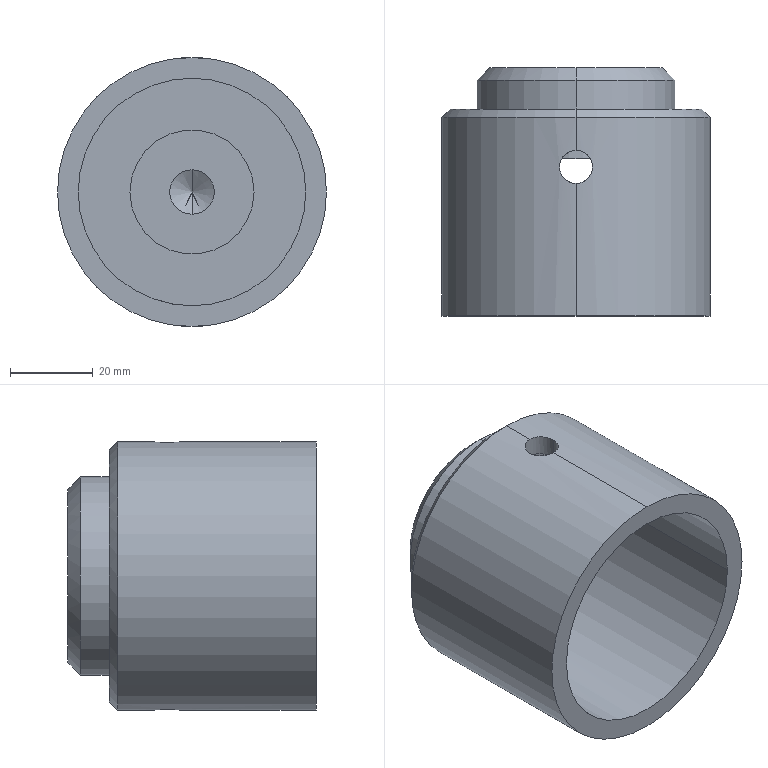Part | SolidWorks | features Chamfer 2, ICE 2, RevCut 2, Revolution 1 | 1 solid | 25 faces | box 65 x 60 x 65 mm | volume 87654 mm3 | cylinder 14 | cone 6 | plane 5 | commonest cylinder face diameters 8 x4 10.75 x2 30 x2 48 x2 55 x2 65 x2
STEP:
#1=CARTESIAN_POINT('',(0.,38.,-5.375));
#2=VERTEX_POINT('',#1);
#3=CARTESIAN_POINT('',(0.,38.,5.375));
#4=VERTEX_POINT('',#3);
#5=CARTESIAN_POINT('',(0.,38.,0.));
#6=DIRECTION('',(0.,1.,0.));
#7=DIRECTION('',(0.,0.,1.));
#8=AXIS2_PLACEMENT_3D('',#5,#6,#7);
#9=CIRCLE('',#8,5.375);
#10=EDGE_CURVE('',#2,#4,#9,.T.);
#11=ORIENTED_EDGE('',*,*,#10,.F.);
#12=CARTESIAN_POINT('',(0.,50.,-5.375));
#13=VERTEX_POINT('',#12);
#14=CARTESIAN_POINT('',(0.,53.103,-5.375));
#15=DIRECTION('',(0.,1.,0.));
#16=VECTOR('',#15,1000.);
#17=LINE('',#14,#16);
#18=EDGE_CURVE('',#2,#13,#17,.T.);
#19=ORIENTED_EDGE('',*,*,#18,.T.);
#20=CARTESIAN_POINT('',(0.,50.,5.375));
#21=VERTEX_POINT('',#20);
#22=CARTESIAN_POINT('',(0.,50.,0.));
#23=DIRECTION('',(0.,1.,0.));
#24=DIRECTION('',(0.,0.,1.));
#25=AXIS2_PLACEMENT_3D('',#22,#23,#24);
#26=CIRCLE('',#25,5.375);
#27=EDGE_CURVE('',#13,#21,#26,.T.);
#28=ORIENTED_EDGE('',*,*,#27,.T.);
#29=CARTESIAN_POINT('',(0.,53.103,5.375));
#30=DIRECTION('',(0.,1.,0.));
#31=VECTOR('',#30,1000.);
#32=LINE('',#29,#31);
#33=EDGE_CURVE('',#4,#21,#32,.T.);
#34=ORIENTED_EDGE('',*,*,#33,.F.);
#35=EDGE_LOOP('',(#11,#19,#28,#34));
#36=FACE_OUTER_BOUND('',#35,.T.);
#37=CARTESIAN_POINT('',(0.,53.103,0.));
#38=DIRECTION('',(0.,1.,0.));
#39=DIRECTION('',(0.,0.,1.));
#40=AXIS2_PLACEMENT_3D('',#37,#38,#39);
#41=CYLINDRICAL_SURFACE('',#40,5.375);
#42=ADVANCED_FACE('',(#36),#41,.F.);
#43=CARTESIAN_POINT('',(0.,53.103,0.));
#44=VERTEX_POINT('',#43);
#45=CARTESIAN_POINT('',(0.,53.103,0.));
#46=DIRECTION('',(0.,-0.5,-0.866));
#47=VECTOR('',#46,1000.);
#48=LINE('',#45,#47);
#49=EDGE_CURVE('',#44,#13,#48,.T.);
#50=ORIENTED_EDGE('',*,*,#49,.F.);
#51=CARTESIAN_POINT('',(0.,53.103,0.));
#52=DIRECTION('',(0.,-0.5,0.866));
#53=VECTOR('',#52,1000.);
#54=LINE('',#51,#53);
#55=EDGE_CURVE('',#44,#21,#54,.T.);
#56=ORIENTED_EDGE('',*,*,#55,.T.);
#57=ORIENTED_EDGE('',*,*,#27,.F.);
#58=EDGE_LOOP('',(#50,#56,#57));
#59=FACE_OUTER_BOUND('',#58,.T.);
#60=CARTESIAN_POINT('',(0.,-946.897,0.));
#61=DIRECTION('',(0.,-1.,0.));
#62=DIRECTION('',(0.,0.,-1.));
#63=AXIS2_PLACEMENT_3D('',#60,#61,#62);
#64=CONICAL_SURFACE('',#63,1732.051,1.047);
#65=ADVANCED_FACE('',(#59),#64,.F.);
#66=CARTESIAN_POINT('',(0.,32.,32.5));
#67=VERTEX_POINT('',#66);
#68=CARTESIAN_POINT('',(4.,36.,32.253));
#69=VERTEX_POINT('',#68);
#70=CARTESIAN_POINT('',(0.,32.,32.5));
#71=CARTESIAN_POINT('',(0.2611,32.,32.5));
#72=CARTESIAN_POINT('',(0.5264,32.026,32.497));
#73=CARTESIAN_POINT('',(1.039,32.129,32.484));
#74=CARTESIAN_POINT('',(1.289,32.204,32.475));
#75=CARTESIAN_POINT('',(1.773,32.405,32.452));
#76=CARTESIAN_POINT('',(2.007,32.53,32.439));
#77=CARTESIAN_POINT('',(2.44,32.82,32.409));
#78=CARTESIAN_POINT('',(2.642,32.985,32.393));
#79=CARTESIAN_POINT('',(3.015,33.358,32.36));
#80=CARTESIAN_POINT('',(3.18,33.56,32.344));
#81=CARTESIAN_POINT('',(3.47,33.993,32.315));
#82=CARTESIAN_POINT('',(3.595,34.227,32.301));
#83=CARTESIAN_POINT('',(3.796,34.711,32.278));
#84=CARTESIAN_POINT('',(3.871,34.961,32.269));
#85=CARTESIAN_POINT('',(3.974,35.474,32.256));
#86=CARTESIAN_POINT('',(4.,35.739,32.253));
#87=CARTESIAN_POINT('',(4.,36.,32.253));
#88=B_SPLINE_CURVE_WITH_KNOTS('',3,(#70,#71,#72,#73,#74,#75,#76,#77,#78,#79,#80,#81,#82,#83,#84,#85,#86,#87),.UNSPECIFIED.,.F.,.F.,(4,2,2,2,2,2,2,2,4),(0.00626,0.007042,0.007825,0.008607,0.009389,0.01017,0.01095,0.01174,0.01252),.UNSPECIFIED.);
#89=EDGE_CURVE('',#67,#69,#88,.T.);
#90=ORIENTED_EDGE('',*,*,#89,.T.);
#91=CARTESIAN_POINT('',(4.,36.,27.208));
#92=VERTEX_POINT('',#91);
#93=CARTESIAN_POINT('',(4.,36.,125.));
#94=DIRECTION('',(0.,0.,-1.));
#95=VECTOR('',#94,1000.);
#96=LINE('',#93,#95);
#97=EDGE_CURVE('',#69,#92,#96,.T.);
#98=ORIENTED_EDGE('',*,*,#97,.T.);
#99=CARTESIAN_POINT('',(-4.,36.,27.208));
#100=VERTEX_POINT('',#99);
#101=CARTESIAN_POINT('',(4.,36.,27.208));
#102=CARTESIAN_POINT('',(4.,35.739,27.208));
#103=CARTESIAN_POINT('',(3.974,35.473,27.211));
#104=CARTESIAN_POINT('',(3.871,34.96,27.226));
#105=CARTESIAN_POINT('',(3.796,34.711,27.237));
#106=CARTESIAN_POINT('',(3.595,34.226,27.264));
#107=CARTESIAN_POINT('',(3.469,33.992,27.281));
#108=CARTESIAN_POINT('',(3.18,33.559,27.316));
#109=CARTESIAN_POINT('',(3.014,33.357,27.335));
#110=CARTESIAN_POINT('',(2.641,32.984,27.374));
#111=CARTESIAN_POINT('',(2.439,32.819,27.392));
#112=CARTESIAN_POINT('',(2.006,32.53,27.428));
#113=CARTESIAN_POINT('',(1.772,32.404,27.444));
#114=CARTESIAN_POINT('',(1.288,32.204,27.471));
#115=CARTESIAN_POINT('',(1.039,32.128,27.482));
#116=CARTESIAN_POINT('',(0.5253,32.026,27.496));
#117=CARTESIAN_POINT('',(0.2599,32.,27.5));
#118=CARTESIAN_POINT('',(-0.2625,32.,27.5));
#119=CARTESIAN_POINT('',(-0.5224,32.026,27.496));
#120=CARTESIAN_POINT('',(-1.039,32.128,27.482));
#121=CARTESIAN_POINT('',(-1.291,32.205,27.471));
#122=CARTESIAN_POINT('',(-1.773,32.405,27.444));
#123=CARTESIAN_POINT('',(-2.006,32.529,27.428));
#124=CARTESIAN_POINT('',(-2.442,32.821,27.392));
#125=CARTESIAN_POINT('',(-2.644,32.987,27.373));
#126=CARTESIAN_POINT('',(-3.012,33.355,27.335));
#127=CARTESIAN_POINT('',(-3.181,33.561,27.316));
#128=CARTESIAN_POINT('',(-3.471,33.995,27.28));
#129=CARTESIAN_POINT('',(-3.594,34.225,27.264));
#130=CARTESIAN_POINT('',(-3.795,34.709,27.237));
#131=CARTESIAN_POINT('',(-3.872,34.963,27.226));
#132=CARTESIAN_POINT('',(-3.974,35.475,27.211));
#133=CARTESIAN_POINT('',(-4.,35.736,27.208));
#134=CARTESIAN_POINT('',(-4.,36.,27.208));
#135=B_SPLINE_CURVE_WITH_KNOTS('',3,(#101,#102,#103,#104,#105,#106,#107,#108,#109,#110,#111,#112,#113,#114,#115,#116,#117,#118,#119,#120,#121,#122,#123,#124,#125,#126,#127,#128,#129,#130,#131,#132,#133,#134),.UNSPECIFIED.,.F.,.F.,(4,2,2,2,2,2,2,2,2,2,2,2,2,2,2,2,4),(0.006263,0.007045,0.007828,0.008611,0.009393,0.01018,0.01096,0.01174,0.01252,0.01331,0.01409,0.01487,0.01565,0.01644,0.01722,0.018,0.01878),.UNSPECIFIED.);
#136=EDGE_CURVE('',#92,#100,#135,.T.);
#137=ORIENTED_EDGE('',*,*,#136,.T.);
#138=CARTESIAN_POINT('',(-4.,36.,32.253));
#139=VERTEX_POINT('',#138);
#140=CARTESIAN_POINT('',(-4.,36.,125.));
#141=DIRECTION('',(0.,0.,-1.));
#142=VECTOR('',#141,1000.);
#143=LINE('',#140,#142);
#144=EDGE_CURVE('',#139,#100,#143,.T.);
#145=ORIENTED_EDGE('',*,*,#144,.F.);
#146=CARTESIAN_POINT('',(-4.,36.,32.253));
#147=CARTESIAN_POINT('',(-4.,35.735,32.253));
#148=CARTESIAN_POINT('',(-3.974,35.475,32.256));
#149=CARTESIAN_POINT('',(-3.872,34.964,32.269));
#150=CARTESIAN_POINT('',(-3.795,34.709,32.278));
#151=CARTESIAN_POINT('',(-3.594,34.225,32.301));
#152=CARTESIAN_POINT('',(-3.471,33.995,32.314));
#153=CARTESIAN_POINT('',(-3.181,33.56,32.344));
#154=CARTESIAN_POINT('',(-3.012,33.355,32.361));
#155=CARTESIAN_POINT('',(-2.643,32.986,32.393));
#156=CARTESIAN_POINT('',(-2.442,32.821,32.409));
#157=CARTESIAN_POINT('',(-2.004,32.528,32.439));
#158=CARTESIAN_POINT('',(-1.772,32.404,32.453));
#159=CARTESIAN_POINT('',(-1.29,32.205,32.475));
#160=CARTESIAN_POINT('',(-1.038,32.128,32.484));
#161=CARTESIAN_POINT('',(-0.521,32.025,32.497));
#162=CARTESIAN_POINT('',(-0.2612,32.,32.5));
#163=CARTESIAN_POINT('',(0.,32.,32.5));
#164=B_SPLINE_CURVE_WITH_KNOTS('',3,(#146,#147,#148,#149,#150,#151,#152,#153,#154,#155,#156,#157,#158,#159,#160,#161,#162,#163),.UNSPECIFIED.,.F.,.F.,(4,2,2,2,2,2,2,2,4),(0.,0.0007825,0.001565,0.002348,0.00313,0.003913,0.004695,0.005478,0.00626),.UNSPECIFIED.);
#165=EDGE_CURVE('',#139,#67,#164,.T.);
#166=ORIENTED_EDGE('',*,*,#165,.T.);
#167=EDGE_LOOP('',(#90,#98,#137,#145,#166));
#168=FACE_OUTER_BOUND('',#167,.T.);
#169=CARTESIAN_POINT('',(0.,36.,125.));
#170=DIRECTION('',(0.,0.,-1.));
#171=DIRECTION('',(-1.,0.,0.));
#172=AXIS2_PLACEMENT_3D('',#169,#170,#171);
#173=CYLINDRICAL_SURFACE('',#172,4.);
#174=ADVANCED_FACE('',(#168),#173,.F.);
#175=CARTESIAN_POINT('',(-4.,36.,-32.253));
#176=VERTEX_POINT('',#175);
#177=CARTESIAN_POINT('',(0.,32.,-32.5));
#178=VERTEX_POINT('',#177);
#179=CARTESIAN_POINT('',(-4.,36.,-32.253));
#180=CARTESIAN_POINT('',(-4.,35.739,-32.253));
#181=CARTESIAN_POINT('',(-3.974,35.474,-32.256));
#182=CARTESIAN_POINT('',(-3.871,34.961,-32.269));
#183=CARTESIAN_POINT('',(-3.796,34.711,-32.278));
#184=CARTESIAN_POINT('',(-3.595,34.227,-32.301));
#185=CARTESIAN_POINT('',(-3.47,33.993,-32.315));
#186=CARTESIAN_POINT('',(-3.18,33.56,-32.344));
#187=CARTESIAN_POINT('',(-3.015,33.358,-32.36));
#188=CARTESIAN_POINT('',(-2.642,32.985,-32.393));
#189=CARTESIAN_POINT('',(-2.44,32.82,-32.409));
#190=CARTESIAN_POINT('',(-2.007,32.53,-32.439));
#191=CARTESIAN_POINT('',(-1.773,32.405,-32.453));
#192=CARTESIAN_POINT('',(-1.289,32.204,-32.475));
#193=CARTESIAN_POINT('',(-1.039,32.129,-32.484));
#194=CARTESIAN_POINT('',(-0.5264,32.026,-32.497));
#195=CARTESIAN_POINT('',(-0.2611,32.,-32.5));
#196=CARTESIAN_POINT('',(0.,32.,-32.5));
#197=B_SPLINE_CURVE_WITH_KNOTS('',3,(#179,#180,#181,#182,#183,#184,#185,#186,#187,#188,#189,#190,#191,#192,#193,#194,#195,#196),.UNSPECIFIED.,.F.,.F.,(4,2,2,2,2,2,2,2,4),(0.00626,0.007042,0.007825,0.008607,0.009389,0.01017,0.01095,0.01174,0.01252),.UNSPECIFIED.);
#198=EDGE_CURVE('',#176,#178,#197,.T.);
#199=ORIENTED_EDGE('',*,*,#198,.F.);
#200=CARTESIAN_POINT('',(-4.,36.,-27.208));
#201=VERTEX_POINT('',#200);
#202=CARTESIAN_POINT('',(-4.,36.,-125.));
#203=DIRECTION('',(0.,0.,1.));
#204=VECTOR('',#203,1000.);
#205=LINE('',#202,#204);
#206=EDGE_CURVE('',#176,#201,#205,.T.);
#207=ORIENTED_EDGE('',*,*,#206,.T.);
#208=CARTESIAN_POINT('',(4.,36.,-27.208));
#209=VERTEX_POINT('',#208);
#210=CARTESIAN_POINT('',(4.,36.,-27.208));
#211=CARTESIAN_POINT('',(4.,35.739,-27.208));
#212=CARTESIAN_POINT('',(3.974,35.473,-27.211));
#213=CARTESIAN_POINT('',(3.871,34.96,-27.226));
#214=CARTESIAN_POINT('',(3.796,34.711,-27.237));
#215=CARTESIAN_POINT('',(3.595,34.226,-27.264));
#216=CARTESIAN_POINT('',(3.469,33.992,-27.281));
#217=CARTESIAN_POINT('',(3.18,33.559,-27.316));
#218=CARTESIAN_POINT('',(3.014,33.357,-27.335));
#219=CARTESIAN_POINT('',(2.641,32.984,-27.374));
#220=CARTESIAN_POINT('',(2.439,32.819,-27.392));
#221=CARTESIAN_POINT('',(2.006,32.53,-27.428));
#222=CARTESIAN_POINT('',(1.772,32.404,-27.444));
#223=CARTESIAN_POINT('',(1.288,32.204,-27.471));
#224=CARTESIAN_POINT('',(1.039,32.128,-27.482));
#225=CARTESIAN_POINT('',(0.5253,32.026,-27.496));
#226=CARTESIAN_POINT('',(0.2599,32.,-27.5));
#227=CARTESIAN_POINT('',(-0.2625,32.,-27.5));
#228=CARTESIAN_POINT('',(-0.5224,32.026,-27.496));
#229=CARTESIAN_POINT('',(-1.039,32.128,-27.482));
#230=CARTESIAN_POINT('',(-1.291,32.205,-27.471));
#231=CARTESIAN_POINT('',(-1.773,32.405,-27.444));
#232=CARTESIAN_POINT('',(-2.006,32.529,-27.428));
#233=CARTESIAN_POINT('',(-2.442,32.821,-27.392));
#234=CARTESIAN_POINT('',(-2.644,32.987,-27.373));
#235=CARTESIAN_POINT('',(-3.012,33.355,-27.335));
#236=CARTESIAN_POINT('',(-3.181,33.561,-27.316));
#237=CARTESIAN_POINT('',(-3.471,33.995,-27.28));
#238=CARTESIAN_POINT('',(-3.594,34.225,-27.264));
#239=CARTESIAN_POINT('',(-3.795,34.709,-27.237));
#240=CARTESIAN_POINT('',(-3.872,34.963,-27.226));
#241=CARTESIAN_POINT('',(-3.974,35.475,-27.211));
#242=CARTESIAN_POINT('',(-4.,35.736,-27.208));
#243=CARTESIAN_POINT('',(-4.,36.,-27.208));
#244=B_SPLINE_CURVE_WITH_KNOTS('',3,(#210,#211,#212,#213,#214,#215,#216,#217,#218,#219,#220,#221,#222,#223,#224,#225,#226,#227,#228,#229,#230,#231,#232,#233,#234,#235,#236,#237,#238,#239,#240,#241,#242,#243),.UNSPECIFIED.,.F.,.F.,(4,2,2,2,2,2,2,2,2,2,2,2,2,2,2,2,4),(0.006263,0.007045,0.007828,0.008611,0.009393,0.01018,0.01096,0.01174,0.01252,0.01331,0.01409,0.01487,0.01565,0.01644,0.01722,0.018,0.01878),.UNSPECIFIED.);
#245=EDGE_CURVE('',#209,#201,#244,.T.);
#246=ORIENTED_EDGE('',*,*,#245,.F.);
#247=CARTESIAN_POINT('',(4.,36.,-32.253));
#248=VERTEX_POINT('',#247);
#249=CARTESIAN_POINT('',(4.,36.,-125.));
#250=DIRECTION('',(0.,0.,1.));
#251=VECTOR('',#250,1000.);
#252=LINE('',#249,#251);
#253=EDGE_CURVE('',#248,#209,#252,.T.);
#254=ORIENTED_EDGE('',*,*,#253,.F.);
#255=CARTESIAN_POINT('',(0.,32.,-32.5));
#256=CARTESIAN_POINT('',(0.2612,32.,-32.5));
#257=CARTESIAN_POINT('',(0.5211,32.025,-32.497));
#258=CARTESIAN_POINT('',(1.038,32.128,-32.484));
#259=CARTESIAN_POINT('',(1.29,32.205,-32.475));
#260=CARTESIAN_POINT('',(1.772,32.404,-32.453));
#261=CARTESIAN_POINT('',(2.005,32.529,-32.439));
#262=CARTESIAN_POINT('',(2.442,32.821,-32.409));
#263=CARTESIAN_POINT('',(2.643,32.986,-32.393));
#264=CARTESIAN_POINT('',(3.012,33.355,-32.361));
#265=CARTESIAN_POINT('',(3.181,33.561,-32.344));
#266=CARTESIAN_POINT('',(3.471,33.995,-32.314));
#267=CARTESIAN_POINT('',(3.594,34.225,-32.301));
#268=CARTESIAN_POINT('',(3.795,34.709,-32.278));
#269=CARTESIAN_POINT('',(3.872,34.964,-32.269));
#270=CARTESIAN_POINT('',(3.974,35.475,-32.256));
#271=CARTESIAN_POINT('',(4.,35.735,-32.253));
#272=CARTESIAN_POINT('',(4.,36.,-32.253));
#273=B_SPLINE_CURVE_WITH_KNOTS('',3,(#255,#256,#257,#258,#259,#260,#261,#262,#263,#264,#265,#266,#267,#268,#269,#270,#271,#272),.UNSPECIFIED.,.F.,.F.,(4,2,2,2,2,2,2,2,4),(0.01252,0.0133,0.01408,0.01487,0.01565,0.01643,0.01721,0.018,0.01878),.UNSPECIFIED.);
#274=EDGE_CURVE('',#178,#248,#273,.T.);
#275=ORIENTED_EDGE('',*,*,#274,.F.);
#276=EDGE_LOOP('',(#199,#207,#246,#254,#275));
#277=FACE_OUTER_BOUND('',#276,.T.);
#278=CARTESIAN_POINT('',(0.,36.,-125.));
#279=DIRECTION('',(0.,0.,1.));
#280=DIRECTION('',(1.,0.,0.));
#281=AXIS2_PLACEMENT_3D('',#278,#279,#280);
#282=CYLINDRICAL_SURFACE('',#281,4.);
#283=ADVANCED_FACE('',(#277),#282,.F.);
#284=CARTESIAN_POINT('',(-15.,38.,0.));
#285=VERTEX_POINT('',#284);
#286=CARTESIAN_POINT('',(15.,38.,0.));
#287=VERTEX_POINT('',#286);
#288=CARTESIAN_POINT('',(0.,38.,0.));
#289=DIRECTION('',(0.,1.,0.));
#290=DIRECTION('',(-1.,0.,0.));
#291=AXIS2_PLACEMENT_3D('',#288,#289,#290);
#292=CIRCLE('',#291,15.);
#293=EDGE_CURVE('',#285,#287,#292,.T.);
#294=ORIENTED_EDGE('',*,*,#293,.T.);
#295=CARTESIAN_POINT('',(15.,40.,0.));
#296=VERTEX_POINT('',#295);
#297=CARTESIAN_POINT('',(15.,38.,0.));
#298=DIRECTION('',(0.,1.,0.));
#299=VECTOR('',#298,1000.);
#300=LINE('',#297,#299);
#301=EDGE_CURVE('',#287,#296,#300,.T.);
#302=ORIENTED_EDGE('',*,*,#301,.T.);
#303=CARTESIAN_POINT('',(-15.,40.,0.));
#304=VERTEX_POINT('',#303);
#305=CARTESIAN_POINT('',(0.,40.,0.));
#306=DIRECTION('',(0.,1.,0.));
#307=DIRECTION('',(-1.,0.,0.));
#308=AXIS2_PLACEMENT_3D('',#305,#306,#307);
#309=CIRCLE('',#308,15.);
#310=EDGE_CURVE('',#304,#296,#309,.T.);
#311=ORIENTED_EDGE('',*,*,#310,.F.);
#312=CARTESIAN_POINT('',(-15.,38.,0.));
#313=DIRECTION('',(0.,1.,0.));
#314=VECTOR('',#313,1000.);
#315=LINE('',#312,#314);
#316=EDGE_CURVE('',#285,#304,#315,.T.);
#317=ORIENTED_EDGE('',*,*,#316,.F.);
#318=EDGE_LOOP('',(#294,#302,#311,#317));
#319=FACE_OUTER_BOUND('',#318,.T.);
#320=CARTESIAN_POINT('',(0.,38.,0.));
#321=DIRECTION('',(0.,1.,0.));
#322=DIRECTION('',(-1.,0.,0.));
#323=AXIS2_PLACEMENT_3D('',#320,#321,#322);
#324=CYLINDRICAL_SURFACE('',#323,15.);
#325=ADVANCED_FACE('',(#319),#324,.T.);
#326=CARTESIAN_POINT('',(0.,50.,30.5));
#327=VERTEX_POINT('',#326);
#328=CARTESIAN_POINT('',(0.,50.,-30.5));
#329=VERTEX_POINT('',#328);
#330=CARTESIAN_POINT('',(0.,50.,0.));
#331=DIRECTION('',(0.,1.,0.));
#332=DIRECTION('',(0.,0.,-1.));
#333=AXIS2_PLACEMENT_3D('',#330,#331,#332);
#334=CIRCLE('',#333,30.5);
#335=EDGE_CURVE('',#327,#329,#334,.T.);
#336=ORIENTED_EDGE('',*,*,#335,.F.);
#337=CARTESIAN_POINT('',(0.,48.,32.5));
#338=VERTEX_POINT('',#337);
#339=CARTESIAN_POINT('',(0.,48.,32.5));
#340=DIRECTION('',(0.,-0.7071,0.7071));
#341=VECTOR('',#340,1000.);
#342=LINE('',#339,#341);
#343=EDGE_CURVE('',#327,#338,#342,.T.);
#344=ORIENTED_EDGE('',*,*,#343,.T.);
#345=CARTESIAN_POINT('',(0.,48.,-32.5));
#346=VERTEX_POINT('',#345);
#347=CARTESIAN_POINT('',(0.,48.,0.));
#348=DIRECTION('',(0.,-1.,0.));
#349=DIRECTION('',(0.,0.,-1.));
#350=AXIS2_PLACEMENT_3D('',#347,#348,#349);
#351=CIRCLE('',#350,32.5);
#352=EDGE_CURVE('',#346,#338,#351,.T.);
#353=ORIENTED_EDGE('',*,*,#352,.F.);
#354=CARTESIAN_POINT('',(0.,48.,-32.5));
#355=DIRECTION('',(0.,-0.7071,-0.7071));
#356=VECTOR('',#355,1000.);
#357=LINE('',#354,#356);
#358=EDGE_CURVE('',#329,#346,#357,.T.);
#359=ORIENTED_EDGE('',*,*,#358,.F.);
#360=EDGE_LOOP('',(#336,#344,#353,#359));
#361=FACE_OUTER_BOUND('',#360,.T.);
#362=CARTESIAN_POINT('',(0.,48.,0.));
#363=DIRECTION('',(0.,-1.,0.));
#364=DIRECTION('',(0.,0.,-1.));
#365=AXIS2_PLACEMENT_3D('',#362,#363,#364);
#366=CONICAL_SURFACE('',#365,32.5,0.7854);
#367=ADVANCED_FACE('',(#361),#366,.T.);
#368=CARTESIAN_POINT('',(0.,60.,21.));
#369=VERTEX_POINT('',#368);
#370=CARTESIAN_POINT('',(0.,60.,-21.));
#371=VERTEX_POINT('',#370);
#372=CARTESIAN_POINT('',(0.,60.,0.));
#373=DIRECTION('',(0.,1.,0.));
#374=DIRECTION('',(0.,0.,-1.));
#375=AXIS2_PLACEMENT_3D('',#372,#373,#374);
#376=CIRCLE('',#375,21.);
#377=EDGE_CURVE('',#369,#371,#376,.T.);
#378=ORIENTED_EDGE('',*,*,#377,.F.);
#379=CARTESIAN_POINT('',(0.,57.,24.));
#380=VERTEX_POINT('',#379);
#381=CARTESIAN_POINT('',(0.,57.,24.));
#382=DIRECTION('',(0.,-0.7071,0.7071));
#383=VECTOR('',#382,1000.);
#384=LINE('',#381,#383);
#385=EDGE_CURVE('',#369,#380,#384,.T.);
#386=ORIENTED_EDGE('',*,*,#385,.T.);
#387=CARTESIAN_POINT('',(0.,57.,-24.));
#388=VERTEX_POINT('',#387);
#389=CARTESIAN_POINT('',(0.,57.,0.));
#390=DIRECTION('',(0.,-1.,0.));
#391=DIRECTION('',(0.,0.,-1.));
#392=AXIS2_PLACEMENT_3D('',#389,#390,#391);
#393=CIRCLE('',#392,24.);
#394=EDGE_CURVE('',#388,#380,#393,.T.);
#395=ORIENTED_EDGE('',*,*,#394,.F.);
#396=CARTESIAN_POINT('',(0.,57.,-24.));
#397=DIRECTION('',(0.,-0.7071,-0.7071));
#398=VECTOR('',#397,1000.);
#399=LINE('',#396,#398);
#400=EDGE_CURVE('',#371,#388,#399,.T.);
#401=ORIENTED_EDGE('',*,*,#400,.F.);
#402=EDGE_LOOP('',(#378,#386,#395,#401));
#403=FACE_OUTER_BOUND('',#402,.T.);
#404=CARTESIAN_POINT('',(0.,57.,0.));
#405=DIRECTION('',(0.,-1.,0.));
#406=DIRECTION('',(0.,0.,-1.));
#407=AXIS2_PLACEMENT_3D('',#404,#405,#406);
#408=CONICAL_SURFACE('',#407,24.,0.7854);
#409=ADVANCED_FACE('',(#403),#408,.T.);
#410=ORIENTED_EDGE('',*,*,#394,.T.);
#411=CARTESIAN_POINT('',(0.,50.,24.));
#412=VERTEX_POINT('',#411);
#413=CARTESIAN_POINT('',(0.,0.,24.));
#414=DIRECTION('',(0.,-1.,0.));
#415=VECTOR('',#414,1000.);
#416=LINE('',#413,#415);
#417=EDGE_CURVE('',#380,#412,#416,.T.);
#418=ORIENTED_EDGE('',*,*,#417,.T.);
#419=CARTESIAN_POINT('',(0.,50.,-24.));
#420=VERTEX_POINT('',#419);
#421=CARTESIAN_POINT('',(0.,50.,0.));
#422=DIRECTION('',(0.,-1.,0.));
#423=DIRECTION('',(0.,0.,-1.));
#424=AXIS2_PLACEMENT_3D('',#421,#422,#423);
#425=CIRCLE('',#424,24.);
#426=EDGE_CURVE('',#420,#412,#425,.T.);
#427=ORIENTED_EDGE('',*,*,#426,.F.);
#428=CARTESIAN_POINT('',(0.,0.,-24.));
#429=DIRECTION('',(0.,-1.,0.));
#430=VECTOR('',#429,1000.);
#431=LINE('',#428,#430);
#432=EDGE_CURVE('',#388,#420,#431,.T.);
#433=ORIENTED_EDGE('',*,*,#432,.F.);
#434=EDGE_LOOP('',(#410,#418,#427,#433));
#435=FACE_OUTER_BOUND('',#434,.T.);
#436=CARTESIAN_POINT('',(0.,0.,0.));
#437=DIRECTION('',(0.,-1.,0.));
#438=DIRECTION('',(0.,0.,-1.));
#439=AXIS2_PLACEMENT_3D('',#436,#437,#438);
#440=CYLINDRICAL_SURFACE('',#439,24.);
#441=ADVANCED_FACE('',(#435),#440,.T.);
#442=CARTESIAN_POINT('',(27.5,0.,0.));
#443=VERTEX_POINT('',#442);
#444=CARTESIAN_POINT('',(-27.5,0.,0.));
#445=VERTEX_POINT('',#444);
#446=CARTESIAN_POINT('',(0.,0.,0.));
#447=DIRECTION('',(0.,1.,0.));
#448=DIRECTION('',(-1.,0.,0.));
#449=AXIS2_PLACEMENT_3D('',#446,#447,#448);
#450=CIRCLE('',#449,27.5);
#451=EDGE_CURVE('',#443,#445,#450,.T.);
#452=ORIENTED_EDGE('',*,*,#451,.F.);
#453=CARTESIAN_POINT('',(27.5,40.,0.));
#454=VERTEX_POINT('',#453);
#455=CARTESIAN_POINT('',(27.5,38.,0.));
#456=DIRECTION('',(0.,1.,0.));
#457=VECTOR('',#456,1000.);
#458=LINE('',#455,#457);
#459=EDGE_CURVE('',#443,#454,#458,.T.);
#460=ORIENTED_EDGE('',*,*,#459,.T.);
#461=CARTESIAN_POINT('',(0.,40.,-27.5));
#462=VERTEX_POINT('',#461);
#463=CARTESIAN_POINT('',(0.,40.,0.));
#464=DIRECTION('',(0.,1.,0.));
#465=DIRECTION('',(-1.,0.,0.));
#466=AXIS2_PLACEMENT_3D('',#463,#464,#465);
#467=CIRCLE('',#466,27.5);
#468=EDGE_CURVE('',#454,#462,#467,.T.);
#469=ORIENTED_EDGE('',*,*,#468,.T.);
#470=CARTESIAN_POINT('',(0.,40.,-27.5));
#471=CARTESIAN_POINT('',(0.2647,40.,-27.5));
#472=CARTESIAN_POINT('',(0.525,39.974,-27.496));
#473=CARTESIAN_POINT('',(1.037,39.872,-27.482));
#474=CARTESIAN_POINT('',(1.291,39.795,-27.471));
#475=CARTESIAN_POINT('',(1.776,39.594,-27.444));
#476=CARTESIAN_POINT('',(2.005,39.471,-27.428));
#477=CARTESIAN_POINT('',(2.44,39.18,-27.392));
#478=CARTESIAN_POINT('',(2.645,39.012,-27.373));
#479=CARTESIAN_POINT('',(3.014,38.643,-27.335));
#480=CARTESIAN_POINT('',(3.179,38.442,-27.316));
#481=CARTESIAN_POINT('',(3.472,38.004,-27.28));
#482=CARTESIAN_POINT('',(3.596,37.772,-27.264));
#483=CARTESIAN_POINT('',(3.795,37.29,-27.237));
#484=CARTESIAN_POINT('',(3.872,37.038,-27.226));
#485=CARTESIAN_POINT('',(3.975,36.521,-27.211));
#486=CARTESIAN_POINT('',(4.,36.261,-27.208));
#487=CARTESIAN_POINT('',(4.,36.,-27.208));
#488=B_SPLINE_CURVE_WITH_KNOTS('',3,(#470,#471,#472,#473,#474,#475,#476,#477,#478,#479,#480,#481,#482,#483,#484,#485,#486,#487),.UNSPECIFIED.,.F.,.F.,(4,2,2,2,2,2,2,2,4),(0.,0.0007828,0.001566,0.002349,0.003131,0.003914,0.004697,0.00548,0.006263),.UNSPECIFIED.);
#489=EDGE_CURVE('',#462,#209,#488,.T.);
#490=ORIENTED_EDGE('',*,*,#489,.T.);
#491=ORIENTED_EDGE('',*,*,#245,.T.);
#492=CARTESIAN_POINT('',(-4.,36.,-27.208));
#493=CARTESIAN_POINT('',(-4.,36.264,-27.208));
#494=CARTESIAN_POINT('',(-3.974,36.524,-27.211));
#495=CARTESIAN_POINT('',(-3.872,37.036,-27.226));
#496=CARTESIAN_POINT('',(-3.795,37.29,-27.237));
#497=CARTESIAN_POINT('',(-3.595,37.774,-27.264));
#498=CARTESIAN_POINT('',(-3.472,38.003,-27.28));
#499=CARTESIAN_POINT('',(-3.182,38.438,-27.316));
#500=CARTESIAN_POINT('',(-3.013,38.643,-27.335));
#501=CARTESIAN_POINT('',(-2.645,39.012,-27.373));
#502=CARTESIAN_POINT('',(-2.444,39.177,-27.392));
#503=CARTESIAN_POINT('',(-2.007,39.47,-27.428));
#504=CARTESIAN_POINT('',(-1.776,39.594,-27.444));
#505=CARTESIAN_POINT('',(-1.295,39.794,-27.471));
#506=CARTESIAN_POINT('',(-1.043,39.871,-27.481));
#507=CARTESIAN_POINT('',(-0.5259,39.974,-27.496));
#508=CARTESIAN_POINT('',(-0.2645,40.,-27.5));
#509=CARTESIAN_POINT('',(0.,40.,-27.5));
#510=B_SPLINE_CURVE_WITH_KNOTS('',3,(#492,#493,#494,#495,#496,#497,#498,#499,#500,#501,#502,#503,#504,#505,#506,#507,#508,#509),.UNSPECIFIED.,.F.,.F.,(4,2,2,2,2,2,2,2,4),(0.01878,0.01957,0.02035,0.02113,0.02191,0.0227,0.02348,0.02426,0.02504),.UNSPECIFIED.);
#511=EDGE_CURVE('',#201,#462,#510,.T.);
#512=ORIENTED_EDGE('',*,*,#511,.T.);
#513=CARTESIAN_POINT('',(-27.5,40.,0.));
#514=VERTEX_POINT('',#513);
#515=CARTESIAN_POINT('',(0.,40.,0.));
#516=DIRECTION('',(0.,1.,0.));
#517=DIRECTION('',(-1.,0.,0.));
#518=AXIS2_PLACEMENT_3D('',#515,#516,#517);
#519=CIRCLE('',#518,27.5);
#520=EDGE_CURVE('',#462,#514,#519,.T.);
#521=ORIENTED_EDGE('',*,*,#520,.T.);
#522=CARTESIAN_POINT('',(-27.5,38.,0.));
#523=DIRECTION('',(0.,1.,0.));
#524=VECTOR('',#523,1000.);
#525=LINE('',#522,#524);
#526=EDGE_CURVE('',#445,#514,#525,.T.);
#527=ORIENTED_EDGE('',*,*,#526,.F.);
#528=EDGE_LOOP('',(#452,#460,#469,#490,#491,#512,#521,#527));
#529=FACE_OUTER_BOUND('',#528,.T.);
#530=CARTESIAN_POINT('',(0.,38.,0.));
#531=DIRECTION('',(0.,1.,0.));
#532=DIRECTION('',(-1.,0.,0.));
#533=AXIS2_PLACEMENT_3D('',#530,#531,#532);
#534=CYLINDRICAL_SURFACE('',#533,27.5);
#535=ADVANCED_FACE('',(#529),#534,.F.);
#536=ORIENTED_EDGE('',*,*,#352,.T.);
#537=CARTESIAN_POINT('',(0.,40.,32.5));
#538=VERTEX_POINT('',#537);
#539=CARTESIAN_POINT('',(0.,0.,32.5));
#540=DIRECTION('',(0.,-1.,0.));
#541=VECTOR('',#540,1000.);
#542=LINE('',#539,#541);
#543=EDGE_CURVE('',#338,#538,#542,.T.);
#544=ORIENTED_EDGE('',*,*,#543,.T.);
#545=CARTESIAN_POINT('',(4.,36.,32.253));
#546=CARTESIAN_POINT('',(4.,36.261,32.253));
#547=CARTESIAN_POINT('',(3.975,36.521,32.256));
#548=CARTESIAN_POINT('',(3.872,37.038,32.269));
#549=CARTESIAN_POINT('',(3.795,37.29,32.278));
#550=CARTESIAN_POINT('',(3.596,37.772,32.301));
#551=CARTESIAN_POINT('',(3.471,38.005,32.314));
#552=CARTESIAN_POINT('',(3.179,38.442,32.344));
#553=CARTESIAN_POINT('',(3.014,38.643,32.36));
#554=CARTESIAN_POINT('',(2.645,39.012,32.393));
#555=CARTESIAN_POINT('',(2.439,39.181,32.409));
#556=CARTESIAN_POINT('',(2.005,39.471,32.439));
#557=CARTESIAN_POINT('',(1.775,39.594,32.452));
#558=CARTESIAN_POINT('',(1.291,39.795,32.475));
#559=CARTESIAN_POINT('',(1.036,39.872,32.484));
#560=CARTESIAN_POINT('',(0.5248,39.974,32.497));
#561=CARTESIAN_POINT('',(0.2646,40.,32.5));
#562=CARTESIAN_POINT('',(0.,40.,32.5));
#563=B_SPLINE_CURVE_WITH_KNOTS('',3,(#545,#546,#547,#548,#549,#550,#551,#552,#553,#554,#555,#556,#557,#558,#559,#560,#561,#562),.UNSPECIFIED.,.F.,.F.,(4,2,2,2,2,2,2,2,4),(0.01252,0.0133,0.01408,0.01487,0.01565,0.01643,0.01721,0.018,0.01878),.UNSPECIFIED.);
#564=EDGE_CURVE('',#69,#538,#563,.T.);
#565=ORIENTED_EDGE('',*,*,#564,.F.);
#566=ORIENTED_EDGE('',*,*,#89,.F.);
#567=CARTESIAN_POINT('',(0.,0.,32.5));
#568=VERTEX_POINT('',#567);
#569=CARTESIAN_POINT('',(0.,0.,32.5));
#570=DIRECTION('',(0.,-1.,0.));
#571=VECTOR('',#570,1000.);
#572=LINE('',#569,#571);
#573=EDGE_CURVE('',#67,#568,#572,.T.);
#574=ORIENTED_EDGE('',*,*,#573,.T.);
#575=CARTESIAN_POINT('',(0.,0.,-32.5));
#576=VERTEX_POINT('',#575);
#577=CARTESIAN_POINT('',(0.,0.,0.));
#578=DIRECTION('',(0.,-1.,0.));
#579=DIRECTION('',(0.,0.,-1.));
#580=AXIS2_PLACEMENT_3D('',#577,#578,#579);
#581=CIRCLE('',#580,32.5);
#582=EDGE_CURVE('',#576,#568,#581,.T.);
#583=ORIENTED_EDGE('',*,*,#582,.F.);
#584=CARTESIAN_POINT('',(0.,0.,-32.5));
#585=DIRECTION('',(0.,-1.,0.));
#586=VECTOR('',#585,1000.);
#587=LINE('',#584,#586);
#588=EDGE_CURVE('',#178,#576,#587,.T.);
#589=ORIENTED_EDGE('',*,*,#588,.F.);
#590=ORIENTED_EDGE('',*,*,#274,.T.);
#591=CARTESIAN_POINT('',(0.,40.,-32.5));
#592=VERTEX_POINT('',#591);
#593=CARTESIAN_POINT('',(4.,36.,-32.253));
#594=CARTESIAN_POINT('',(4.,36.264,-32.253));
#595=CARTESIAN_POINT('',(3.974,36.524,-32.256));
#596=CARTESIAN_POINT('',(3.872,37.036,-32.269));
#597=CARTESIAN_POINT('',(3.795,37.29,-32.278));
#598=CARTESIAN_POINT('',(3.595,37.774,-32.301));
#599=CARTESIAN_POINT('',(3.472,38.003,-32.314));
#600=CARTESIAN_POINT('',(3.182,38.438,-32.344));
#601=CARTESIAN_POINT('',(3.013,38.643,-32.361));
#602=CARTESIAN_POINT('',(2.645,39.012,-32.393));
#603=CARTESIAN_POINT('',(2.444,39.177,-32.409));
#604=CARTESIAN_POINT('',(2.007,39.47,-32.439));
#605=CARTESIAN_POINT('',(1.775,39.594,-32.452));
#606=CARTESIAN_POINT('',(1.294,39.794,-32.475));
#607=CARTESIAN_POINT('',(1.043,39.871,-32.484));
#608=CARTESIAN_POINT('',(0.5257,39.974,-32.497));
#609=CARTESIAN_POINT('',(0.2644,40.,-32.5));
#610=CARTESIAN_POINT('',(0.,40.,-32.5));
#611=B_SPLINE_CURVE_WITH_KNOTS('',3,(#593,#594,#595,#596,#597,#598,#599,#600,#601,#602,#603,#604,#605,#606,#607,#608,#609,#610),.UNSPECIFIED.,.F.,.F.,(4,2,2,2,2,2,2,2,4),(0.01878,0.01956,0.02034,0.02112,0.02191,0.02269,0.02347,0.02425,0.02503),.UNSPECIFIED.);
#612=EDGE_CURVE('',#248,#592,#611,.T.);
#613=ORIENTED_EDGE('',*,*,#612,.T.);
#614=CARTESIAN_POINT('',(0.,0.,-32.5));
#615=DIRECTION('',(0.,-1.,0.));
#616=VECTOR('',#615,1000.);
#617=LINE('',#614,#616);
#618=EDGE_CURVE('',#346,#592,#617,.T.);
#619=ORIENTED_EDGE('',*,*,#618,.F.);
#620=EDGE_LOOP('',(#536,#544,#565,#566,#574,#583,#589,#590,#613,#619));
#621=FACE_OUTER_BOUND('',#620,.T.);
#622=CARTESIAN_POINT('',(0.,0.,0.));
#623=DIRECTION('',(0.,-1.,0.));
#624=DIRECTION('',(0.,0.,-1.));
#625=AXIS2_PLACEMENT_3D('',#622,#623,#624);
#626=CYLINDRICAL_SURFACE('',#625,32.5);
#627=ADVANCED_FACE('',(#621),#626,.T.);
#628=ORIENTED_EDGE('',*,*,#543,.F.);
#629=CARTESIAN_POINT('',(0.,48.,0.));
#630=DIRECTION('',(0.,-1.,0.));
#631=DIRECTION('',(0.,0.,-1.));
#632=AXIS2_PLACEMENT_3D('',#629,#630,#631);
#633=CIRCLE('',#632,32.5);
#634=EDGE_CURVE('',#338,#346,#633,.T.);
#635=ORIENTED_EDGE('',*,*,#634,.T.);
#636=ORIENTED_EDGE('',*,*,#618,.T.);
#637=CARTESIAN_POINT('',(0.,40.,-32.5));
#638=CARTESIAN_POINT('',(-0.2646,40.,-32.5));
#639=CARTESIAN_POINT('',(-0.5248,39.974,-32.497));
#640=CARTESIAN_POINT('',(-1.036,39.872,-32.484));
#641=CARTESIAN_POINT('',(-1.291,39.795,-32.475));
#642=CARTESIAN_POINT('',(-1.775,39.594,-32.452));
#643=CARTESIAN_POINT('',(-2.005,39.471,-32.439));
#644=CARTESIAN_POINT('',(-2.44,39.181,-32.409));
#645=CARTESIAN_POINT('',(-2.645,39.012,-32.393));
#646=CARTESIAN_POINT('',(-3.014,38.643,-32.36));
#647=CARTESIAN_POINT('',(-3.179,38.442,-32.344));
#648=CARTESIAN_POINT('',(-3.472,38.004,-32.314));
#649=CARTESIAN_POINT('',(-3.596,37.772,-32.301));
#650=CARTESIAN_POINT('',(-3.795,37.29,-32.278));
#651=CARTESIAN_POINT('',(-3.872,37.038,-32.269));
#652=CARTESIAN_POINT('',(-3.975,36.521,-32.256));
#653=CARTESIAN_POINT('',(-4.,36.261,-32.253));
#654=CARTESIAN_POINT('',(-4.,36.,-32.253));
#655=B_SPLINE_CURVE_WITH_KNOTS('',3,(#637,#638,#639,#640,#641,#642,#643,#644,#645,#646,#647,#648,#649,#650,#651,#652,#653,#654),.UNSPECIFIED.,.F.,.F.,(4,2,2,2,2,2,2,2,4),(0.,0.0007825,0.001565,0.002348,0.00313,0.003913,0.004695,0.005478,0.00626),.UNSPECIFIED.);
#656=EDGE_CURVE('',#592,#176,#655,.T.);
#657=ORIENTED_EDGE('',*,*,#656,.T.);
#658=ORIENTED_EDGE('',*,*,#198,.T.);
#659=ORIENTED_EDGE('',*,*,#588,.T.);
#660=CARTESIAN_POINT('',(0.,0.,0.));
#661=DIRECTION('',(0.,-1.,0.));
#662=DIRECTION('',(0.,0.,-1.));
#663=AXIS2_PLACEMENT_3D('',#660,#661,#662);
#664=CIRCLE('',#663,32.5);
#665=EDGE_CURVE('',#568,#576,#664,.T.);
#666=ORIENTED_EDGE('',*,*,#665,.F.);
#667=ORIENTED_EDGE('',*,*,#573,.F.);
#668=ORIENTED_EDGE('',*,*,#165,.F.);
#669=CARTESIAN_POINT('',(0.,40.,32.5));
#670=CARTESIAN_POINT('',(-0.2643,40.,32.5));
#671=CARTESIAN_POINT('',(-0.5242,39.974,32.497));
#672=CARTESIAN_POINT('',(-1.036,39.872,32.485));
#673=CARTESIAN_POINT('',(-1.29,39.795,32.475));
#674=CARTESIAN_POINT('',(-1.774,39.595,32.452));
#675=CARTESIAN_POINT('',(-2.003,39.472,32.439));
#676=CARTESIAN_POINT('',(-2.438,39.182,32.409));
#677=CARTESIAN_POINT('',(-2.643,39.013,32.393));
#678=CARTESIAN_POINT('',(-3.012,38.645,32.361));
#679=CARTESIAN_POINT('',(-3.177,38.444,32.345));
#680=CARTESIAN_POINT('',(-3.47,38.007,32.315));
#681=CARTESIAN_POINT('',(-3.594,37.775,32.301));
#682=CARTESIAN_POINT('',(-3.794,37.294,32.278));
#683=CARTESIAN_POINT('',(-3.871,37.043,32.269));
#684=CARTESIAN_POINT('',(-3.974,36.526,32.256));
#685=CARTESIAN_POINT('',(-4.,36.264,32.253));
#686=CARTESIAN_POINT('',(-4.,36.,32.253));
#687=B_SPLINE_CURVE_WITH_KNOTS('',3,(#669,#670,#671,#672,#673,#674,#675,#676,#677,#678,#679,#680,#681,#682,#683,#684,#685,#686),.UNSPECIFIED.,.F.,.F.,(4,2,2,2,2,2,2,2,4),(0.01878,0.01956,0.02034,0.02112,0.02191,0.02269,0.02347,0.02425,0.02503),.UNSPECIFIED.);
#688=EDGE_CURVE('',#538,#139,#687,.T.);
#689=ORIENTED_EDGE('',*,*,#688,.F.);
#690=EDGE_LOOP('',(#628,#635,#636,#657,#658,#659,#666,#667,#668,#689));
#691=FACE_OUTER_BOUND('',#690,.T.);
#692=CARTESIAN_POINT('',(0.,0.,0.));
#693=DIRECTION('',(0.,-1.,0.));
#694=DIRECTION('',(0.,0.,-1.));
#695=AXIS2_PLACEMENT_3D('',#692,#693,#694);
#696=CYLINDRICAL_SURFACE('',#695,32.5);
#697=ADVANCED_FACE('',(#691),#696,.T.);
#698=ORIENTED_EDGE('',*,*,#459,.F.);
#699=CARTESIAN_POINT('',(0.,0.,0.));
#700=DIRECTION('',(0.,1.,0.));
#701=DIRECTION('',(-1.,0.,0.));
#702=AXIS2_PLACEMENT_3D('',#699,#700,#701);
#703=CIRCLE('',#702,27.5);
#704=EDGE_CURVE('',#445,#443,#703,.T.);
#705=ORIENTED_EDGE('',*,*,#704,.F.);
#706=ORIENTED_EDGE('',*,*,#526,.T.);
#707=CARTESIAN_POINT('',(0.,40.,27.5));
#708=VERTEX_POINT('',#707);
#709=CARTESIAN_POINT('',(0.,40.,0.));
#710=DIRECTION('',(0.,1.,0.));
#711=DIRECTION('',(-1.,0.,0.));
#712=AXIS2_PLACEMENT_3D('',#709,#710,#711);
#713=CIRCLE('',#712,27.5);
#714=EDGE_CURVE('',#514,#708,#713,.T.);
#715=ORIENTED_EDGE('',*,*,#714,.T.);
#716=CARTESIAN_POINT('',(-4.,36.,27.208));
#717=CARTESIAN_POINT('',(-4.,36.264,27.208));
#718=CARTESIAN_POINT('',(-3.974,36.524,27.211));
#719=CARTESIAN_POINT('',(-3.872,37.036,27.226));
#720=CARTESIAN_POINT('',(-3.795,37.29,27.237));
#721=CARTESIAN_POINT('',(-3.595,37.774,27.264));
#722=CARTESIAN_POINT('',(-3.472,38.003,27.28));
#723=CARTESIAN_POINT('',(-3.182,38.438,27.316));
#724=CARTESIAN_POINT('',(-3.013,38.643,27.335));
#725=CARTESIAN_POINT('',(-2.645,39.012,27.373));
#726=CARTESIAN_POINT('',(-2.444,39.177,27.392));
#727=CARTESIAN_POINT('',(-2.007,39.47,27.428));
#728=CARTESIAN_POINT('',(-1.776,39.594,27.444));
#729=CARTESIAN_POINT('',(-1.295,39.794,27.471));
#730=CARTESIAN_POINT('',(-1.043,39.871,27.481));
#731=CARTESIAN_POINT('',(-0.5259,39.974,27.496));
#732=CARTESIAN_POINT('',(-0.2645,40.,27.5));
#733=CARTESIAN_POINT('',(0.,40.,27.5));
#734=B_SPLINE_CURVE_WITH_KNOTS('',3,(#716,#717,#718,#719,#720,#721,#722,#723,#724,#725,#726,#727,#728,#729,#730,#731,#732,#733),.UNSPECIFIED.,.F.,.F.,(4,2,2,2,2,2,2,2,4),(0.01878,0.01957,0.02035,0.02113,0.02191,0.0227,0.02348,0.02426,0.02504),.UNSPECIFIED.);
#735=EDGE_CURVE('',#100,#708,#734,.T.);
#736=ORIENTED_EDGE('',*,*,#735,.F.);
#737=ORIENTED_EDGE('',*,*,#136,.F.);
#738=CARTESIAN_POINT('',(0.,40.,27.5));
#739=CARTESIAN_POINT('',(0.2647,40.,27.5));
#740=CARTESIAN_POINT('',(0.525,39.974,27.496));
#741=CARTESIAN_POINT('',(1.037,39.872,27.482));
#742=CARTESIAN_POINT('',(1.291,39.795,27.471));
#743=CARTESIAN_POINT('',(1.776,39.594,27.444));
#744=CARTESIAN_POINT('',(2.005,39.471,27.428));
#745=CARTESIAN_POINT('',(2.44,39.18,27.392));
#746=CARTESIAN_POINT('',(2.645,39.012,27.373));
#747=CARTESIAN_POINT('',(3.014,38.643,27.335));
#748=CARTESIAN_POINT('',(3.179,38.442,27.316));
#749=CARTESIAN_POINT('',(3.472,38.004,27.28));
#750=CARTESIAN_POINT('',(3.596,37.772,27.264));
#751=CARTESIAN_POINT('',(3.795,37.29,27.237));
#752=CARTESIAN_POINT('',(3.872,37.038,27.226));
#753=CARTESIAN_POINT('',(3.975,36.521,27.211));
#754=CARTESIAN_POINT('',(4.,36.261,27.208));
#755=CARTESIAN_POINT('',(4.,36.,27.208));
#756=B_SPLINE_CURVE_WITH_KNOTS('',3,(#738,#739,#740,#741,#742,#743,#744,#745,#746,#747,#748,#749,#750,#751,#752,#753,#754,#755),.UNSPECIFIED.,.F.,.F.,(4,2,2,2,2,2,2,2,4),(0.,0.0007828,0.001566,0.002349,0.003131,0.003914,0.004697,0.00548,0.006263),.UNSPECIFIED.);
#757=EDGE_CURVE('',#708,#92,#756,.T.);
#758=ORIENTED_EDGE('',*,*,#757,.F.);
#759=CARTESIAN_POINT('',(0.,40.,0.));
#760=DIRECTION('',(0.,1.,0.));
#761=DIRECTION('',(-1.,0.,0.));
#762=AXIS2_PLACEMENT_3D('',#759,#760,#761);
#763=CIRCLE('',#762,27.5);
#764=EDGE_CURVE('',#708,#454,#763,.T.);
#765=ORIENTED_EDGE('',*,*,#764,.T.);
#766=EDGE_LOOP('',(#698,#705,#706,#715,#736,#737,#758,#765));
#767=FACE_OUTER_BOUND('',#766,.T.);
#768=CARTESIAN_POINT('',(0.,38.,0.));
#769=DIRECTION('',(0.,1.,0.));
#770=DIRECTION('',(-1.,0.,0.));
#771=AXIS2_PLACEMENT_3D('',#768,#769,#770);
#772=CYLINDRICAL_SURFACE('',#771,27.5);
#773=ADVANCED_FACE('',(#767),#772,.F.);
#774=CARTESIAN_POINT('',(0.,60.,0.));
#775=DIRECTION('',(0.,1.,0.));
#776=DIRECTION('',(0.,0.,-1.));
#777=AXIS2_PLACEMENT_3D('',#774,#775,#776);
#778=CIRCLE('',#777,21.);
#779=EDGE_CURVE('',#371,#369,#778,.T.);
#780=ORIENTED_EDGE('',*,*,#779,.T.);
#781=ORIENTED_EDGE('',*,*,#377,.T.);
#782=EDGE_LOOP('',(#780,#781));
#783=FACE_OUTER_BOUND('',#782,.T.);
#784=CARTESIAN_POINT('',(0.,60.,0.));
#785=DIRECTION('',(0.,-1.,0.));
#786=DIRECTION('',(0.,0.,-1.));
#787=AXIS2_PLACEMENT_3D('',#784,#785,#786);
#788=PLANE('',#787);
#789=ADVANCED_FACE('',(#783),#788,.F.);
#790=ORIENTED_EDGE('',*,*,#417,.F.);
#791=CARTESIAN_POINT('',(0.,57.,0.));
#792=DIRECTION('',(0.,-1.,0.));
#793=DIRECTION('',(0.,0.,-1.));
#794=AXIS2_PLACEMENT_3D('',#791,#792,#793);
#795=CIRCLE('',#794,24.);
#796=EDGE_CURVE('',#380,#388,#795,.T.);
#797=ORIENTED_EDGE('',*,*,#796,.T.);
#798=ORIENTED_EDGE('',*,*,#432,.T.);
#799=CARTESIAN_POINT('',(0.,50.,0.));
#800=DIRECTION('',(0.,-1.,0.));
#801=DIRECTION('',(0.,0.,-1.));
#802=AXIS2_PLACEMENT_3D('',#799,#800,#801);
#803=CIRCLE('',#802,24.);
#804=EDGE_CURVE('',#412,#420,#803,.T.);
#805=ORIENTED_EDGE('',*,*,#804,.F.);
#806=EDGE_LOOP('',(#790,#797,#798,#805));
#807=FACE_OUTER_BOUND('',#806,.T.);
#808=CARTESIAN_POINT('',(0.,0.,0.));
#809=DIRECTION('',(0.,-1.,0.));
#810=DIRECTION('',(0.,0.,-1.));
#811=AXIS2_PLACEMENT_3D('',#808,#809,#810);
#812=CYLINDRICAL_SURFACE('',#811,24.);
#813=ADVANCED_FACE('',(#807),#812,.T.);
#814=CARTESIAN_POINT('',(0.,50.,0.));
#815=DIRECTION('',(0.,1.,0.));
#816=DIRECTION('',(0.,0.,-1.));
#817=AXIS2_PLACEMENT_3D('',#814,#815,#816);
#818=CIRCLE('',#817,30.5);
#819=EDGE_CURVE('',#329,#327,#818,.T.);
#820=ORIENTED_EDGE('',*,*,#819,.T.);
#821=ORIENTED_EDGE('',*,*,#335,.T.);
#822=EDGE_LOOP('',(#820,#821));
#823=FACE_OUTER_BOUND('',#822,.T.);
#824=ORIENTED_EDGE('',*,*,#426,.T.);
#825=ORIENTED_EDGE('',*,*,#804,.T.);
#826=EDGE_LOOP('',(#824,#825));
#827=FACE_BOUND('',#826,.T.);
#828=CARTESIAN_POINT('',(-24.,50.,0.));
#829=DIRECTION('',(0.,-1.,0.));
#830=DIRECTION('',(0.,0.,-1.));
#831=AXIS2_PLACEMENT_3D('',#828,#829,#830);
#832=PLANE('',#831);
#833=ADVANCED_FACE('',(#823,#827),#832,.F.);
#834=ORIENTED_EDGE('',*,*,#704,.T.);
#835=ORIENTED_EDGE('',*,*,#451,.T.);
#836=EDGE_LOOP('',(#834,#835));
#837=FACE_BOUND('',#836,.T.);
#838=ORIENTED_EDGE('',*,*,#582,.T.);
#839=ORIENTED_EDGE('',*,*,#665,.T.);
#840=EDGE_LOOP('',(#838,#839));
#841=FACE_OUTER_BOUND('',#840,.T.);
#842=CARTESIAN_POINT('',(-32.5,0.,0.));
#843=DIRECTION('',(0.,1.,0.));
#844=DIRECTION('',(0.,0.,1.));
#845=AXIS2_PLACEMENT_3D('',#842,#843,#844);
#846=PLANE('',#845);
#847=ADVANCED_FACE('',(#837,#841),#846,.F.);
#848=ORIENTED_EDGE('',*,*,#385,.F.);
#849=ORIENTED_EDGE('',*,*,#779,.F.);
#850=ORIENTED_EDGE('',*,*,#400,.T.);
#851=ORIENTED_EDGE('',*,*,#796,.F.);
#852=EDGE_LOOP('',(#848,#849,#850,#851));
#853=FACE_OUTER_BOUND('',#852,.T.);
#854=CARTESIAN_POINT('',(0.,57.,0.));
#855=DIRECTION('',(0.,-1.,0.));
#856=DIRECTION('',(0.,0.,-1.));
#857=AXIS2_PLACEMENT_3D('',#854,#855,#856);
#858=CONICAL_SURFACE('',#857,24.,0.7854);
#859=ADVANCED_FACE('',(#853),#858,.T.);
#860=ORIENTED_EDGE('',*,*,#343,.F.);
#861=ORIENTED_EDGE('',*,*,#819,.F.);
#862=ORIENTED_EDGE('',*,*,#358,.T.);
#863=ORIENTED_EDGE('',*,*,#634,.F.);
#864=EDGE_LOOP('',(#860,#861,#862,#863));
#865=FACE_OUTER_BOUND('',#864,.T.);
#866=CARTESIAN_POINT('',(0.,48.,0.));
#867=DIRECTION('',(0.,-1.,0.));
#868=DIRECTION('',(0.,0.,-1.));
#869=AXIS2_PLACEMENT_3D('',#866,#867,#868);
#870=CONICAL_SURFACE('',#869,32.5,0.7854);
#871=ADVANCED_FACE('',(#865),#870,.T.);
#872=ORIENTED_EDGE('',*,*,#764,.F.);
#873=ORIENTED_EDGE('',*,*,#714,.F.);
#874=ORIENTED_EDGE('',*,*,#520,.F.);
#875=ORIENTED_EDGE('',*,*,#468,.F.);
#876=EDGE_LOOP('',(#872,#873,#874,#875));
#877=FACE_OUTER_BOUND('',#876,.T.);
#878=ORIENTED_EDGE('',*,*,#310,.T.);
#879=CARTESIAN_POINT('',(0.,40.,0.));
#880=DIRECTION('',(0.,1.,0.));
#881=DIRECTION('',(-1.,0.,0.));
#882=AXIS2_PLACEMENT_3D('',#879,#880,#881);
#883=CIRCLE('',#882,15.);
#884=EDGE_CURVE('',#296,#304,#883,.T.);
#885=ORIENTED_EDGE('',*,*,#884,.T.);
#886=EDGE_LOOP('',(#878,#885));
#887=FACE_BOUND('',#886,.T.);
#888=CARTESIAN_POINT('',(-27.5,40.,0.));
#889=DIRECTION('',(0.,1.,0.));
#890=DIRECTION('',(-1.,0.,0.));
#891=AXIS2_PLACEMENT_3D('',#888,#889,#890);
#892=PLANE('',#891);
#893=ADVANCED_FACE('',(#877,#887),#892,.F.);
#894=ORIENTED_EDGE('',*,*,#301,.F.);
#895=CARTESIAN_POINT('',(0.,38.,0.));
#896=DIRECTION('',(0.,1.,0.));
#897=DIRECTION('',(-1.,0.,0.));
#898=AXIS2_PLACEMENT_3D('',#895,#896,#897);
#899=CIRCLE('',#898,15.);
#900=EDGE_CURVE('',#287,#285,#899,.T.);
#901=ORIENTED_EDGE('',*,*,#900,.T.);
#902=ORIENTED_EDGE('',*,*,#316,.T.);
#903=ORIENTED_EDGE('',*,*,#884,.F.);
#904=EDGE_LOOP('',(#894,#901,#902,#903));
#905=FACE_OUTER_BOUND('',#904,.T.);
#906=CARTESIAN_POINT('',(0.,38.,0.));
#907=DIRECTION('',(0.,1.,0.));
#908=DIRECTION('',(-1.,0.,0.));
#909=AXIS2_PLACEMENT_3D('',#906,#907,#908);
#910=CYLINDRICAL_SURFACE('',#909,15.);
#911=ADVANCED_FACE('',(#905),#910,.T.);
#912=CARTESIAN_POINT('',(0.,38.,0.));
#913=DIRECTION('',(0.,1.,0.));
#914=DIRECTION('',(0.,0.,1.));
#915=AXIS2_PLACEMENT_3D('',#912,#913,#914);
#916=CIRCLE('',#915,5.375);
#917=EDGE_CURVE('',#4,#2,#916,.T.);
#918=ORIENTED_EDGE('',*,*,#917,.T.);
#919=ORIENTED_EDGE('',*,*,#10,.T.);
#920=EDGE_LOOP('',(#918,#919));
#921=FACE_BOUND('',#920,.T.);
#922=ORIENTED_EDGE('',*,*,#293,.F.);
#923=ORIENTED_EDGE('',*,*,#900,.F.);
#924=EDGE_LOOP('',(#922,#923));
#925=FACE_OUTER_BOUND('',#924,.T.);
#926=CARTESIAN_POINT('',(-15.,38.,0.));
#927=DIRECTION('',(0.,1.,0.));
#928=DIRECTION('',(-1.,0.,0.));
#929=AXIS2_PLACEMENT_3D('',#926,#927,#928);
#930=PLANE('',#929);
#931=ADVANCED_FACE('',(#921,#925),#930,.F.);
#932=ORIENTED_EDGE('',*,*,#206,.F.);
#933=ORIENTED_EDGE('',*,*,#656,.F.);
#934=ORIENTED_EDGE('',*,*,#612,.F.);
#935=ORIENTED_EDGE('',*,*,#253,.T.);
#936=ORIENTED_EDGE('',*,*,#489,.F.);
#937=ORIENTED_EDGE('',*,*,#511,.F.);
#938=EDGE_LOOP('',(#932,#933,#934,#935,#936,#937));
#939=FACE_OUTER_BOUND('',#938,.T.);
#940=CARTESIAN_POINT('',(0.,36.,-125.));
#941=DIRECTION('',(0.,0.,1.));
#942=DIRECTION('',(1.,0.,0.));
#943=AXIS2_PLACEMENT_3D('',#940,#941,#942);
#944=CYLINDRICAL_SURFACE('',#943,4.);
#945=ADVANCED_FACE('',(#939),#944,.F.);
#946=ORIENTED_EDGE('',*,*,#97,.F.);
#947=ORIENTED_EDGE('',*,*,#564,.T.);
#948=ORIENTED_EDGE('',*,*,#688,.T.);
#949=ORIENTED_EDGE('',*,*,#144,.T.);
#950=ORIENTED_EDGE('',*,*,#735,.T.);
#951=ORIENTED_EDGE('',*,*,#757,.T.);
#952=EDGE_LOOP('',(#946,#947,#948,#949,#950,#951));
#953=FACE_OUTER_BOUND('',#952,.T.);
#954=CARTESIAN_POINT('',(0.,36.,125.));
#955=DIRECTION('',(0.,0.,-1.));
#956=DIRECTION('',(-1.,0.,0.));
#957=AXIS2_PLACEMENT_3D('',#954,#955,#956);
#958=CYLINDRICAL_SURFACE('',#957,4.);
#959=ADVANCED_FACE('',(#953),#958,.F.);
#960=ORIENTED_EDGE('',*,*,#55,.F.);
#961=ORIENTED_EDGE('',*,*,#49,.T.);
#962=CARTESIAN_POINT('',(0.,50.,0.));
#963=DIRECTION('',(0.,1.,0.));
#964=DIRECTION('',(0.,0.,1.));
#965=AXIS2_PLACEMENT_3D('',#962,#963,#964);
#966=CIRCLE('',#965,5.375);
#967=EDGE_CURVE('',#21,#13,#966,.T.);
#968=ORIENTED_EDGE('',*,*,#967,.F.);
#969=EDGE_LOOP('',(#960,#961,#968));
#970=FACE_OUTER_BOUND('',#969,.T.);
#971=CARTESIAN_POINT('',(0.,-946.897,0.));
#972=DIRECTION('',(0.,-1.,0.));
#973=DIRECTION('',(0.,0.,-1.));
#974=AXIS2_PLACEMENT_3D('',#971,#972,#973);
#975=CONICAL_SURFACE('',#974,1732.051,1.047);
#976=ADVANCED_FACE('',(#970),#975,.F.);
#977=ORIENTED_EDGE('',*,*,#18,.F.);
#978=ORIENTED_EDGE('',*,*,#917,.F.);
#979=ORIENTED_EDGE('',*,*,#33,.T.);
#980=ORIENTED_EDGE('',*,*,#967,.T.);
#981=EDGE_LOOP('',(#977,#978,#979,#980));
#982=FACE_OUTER_BOUND('',#981,.T.);
#983=CARTESIAN_POINT('',(0.,53.103,0.));
#984=DIRECTION('',(0.,1.,0.));
#985=DIRECTION('',(0.,0.,1.));
#986=AXIS2_PLACEMENT_3D('',#983,#984,#985);
#987=CYLINDRICAL_SURFACE('',#986,5.375);
#988=ADVANCED_FACE('',(#982),#987,.F.);
#989=CLOSED_SHELL('',(#42,#65,#174,#283,#325,#367,#409,#441,#535,#627,#697,#773,#789,#813,#833,#847,#859,#871,#893,#911,#931,#945,#959,#976,#988));
#990=MANIFOLD_SOLID_BREP('',#989);
#991=CARTESIAN_POINT('',(0.,0.,0.));
#992=DIRECTION('',(0.,0.,1.));
#993=DIRECTION('',(1.,0.,0.));
#994=AXIS2_PLACEMENT_3D('',#991,#992,#993);
#995=(LENGTH_UNIT()NAMED_UNIT(*)SI_UNIT(.MILLI.,.METRE.));
#996=UNCERTAINTY_MEASURE_WITH_UNIT(LENGTH_MEASURE(0.00001),#995,'','');
#997=(NAMED_UNIT(*)PLANE_ANGLE_UNIT()SI_UNIT($,.RADIAN.));
#998=(NAMED_UNIT(*)SI_UNIT($,.STERADIAN.)SOLID_ANGLE_UNIT());
#999=(GEOMETRIC_REPRESENTATION_CONTEXT(3)GLOBAL_UNCERTAINTY_ASSIGNED_CONTEXT((#996))GLOBAL_UNIT_ASSIGNED_CONTEXT((#995,#997,#998))REPRESENTATION_CONTEXT('',''));
#1000=ADVANCED_BREP_SHAPE_REPRESENTATION('',(#990,#994),#999);